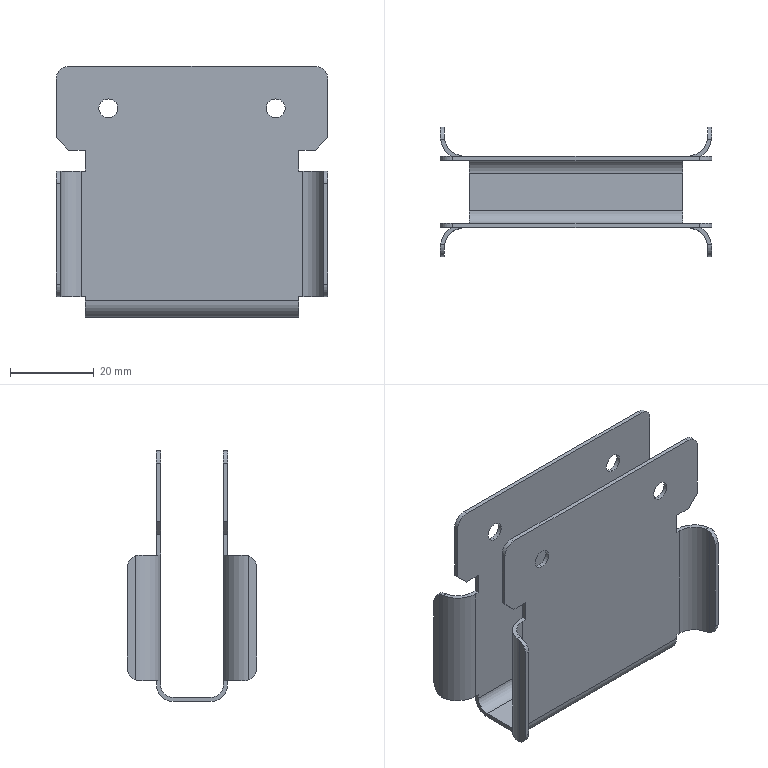Part | SolidWorks | features BaseBody 1 | 1 solid | 78 faces | box 65 x 31 x 60 mm | volume 8584 mm3 | plane 46 | cylinder 32 | commonest cylinder face diameters 6 x14 4.5 x8 10 x4 12 x4 8 x2